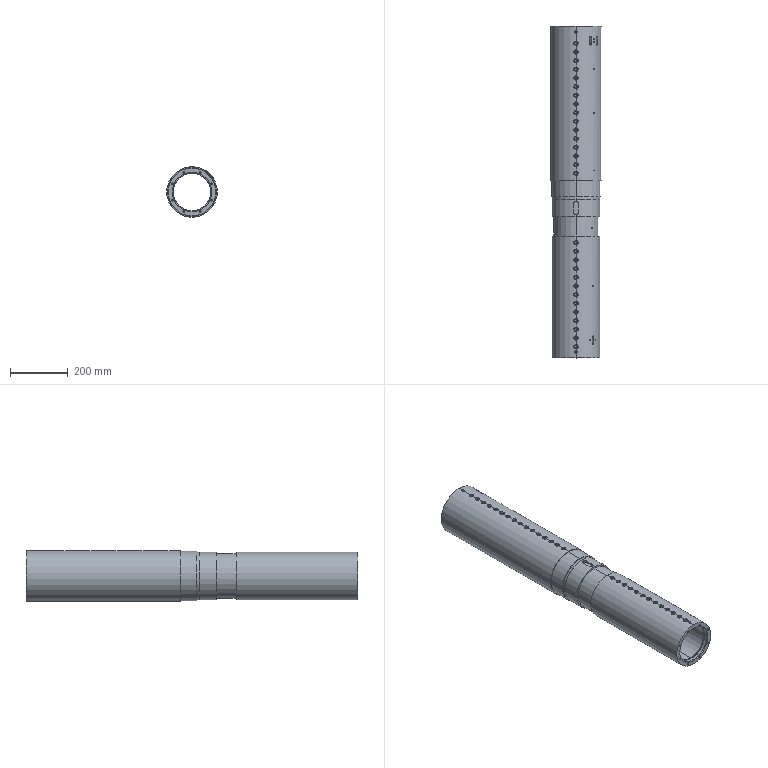Part | SolidWorks | features ICE 9, HoleWzd 7, Chamfer 2, CirPattern 2, Extrusion 1, LPattern 1 | 1 solid | 300 faces | box 175 x 1149 x 175 mm | volume 10647210 mm3 | cylinder 194 | cone 60 | plane 46 | commonest cylinder face diameters 9 x58 15 x58 6.8 x32 3.3 x18 10 x6 8.8 x4